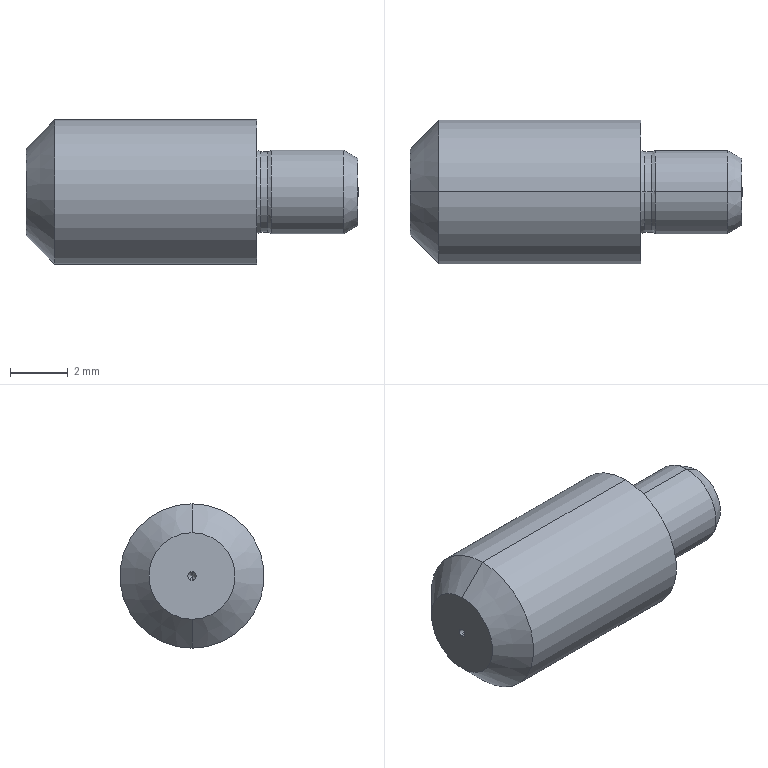Part | STEP file | kfsaph5_p2_90_l8_b3_0_e0_5_a30_2_03 | 1 solid | 21 faces | box 11.5 x 5 x 5 mm | volume 172.579 mm3 | cone 8 | cylinder 6 | spline 4 | plane 3 | commonest cylinder face diameters 2.8 x2 2.9 x2 5 x2
STEP:
#1=CARTESIAN_POINT('',(0.1323,0.,-1.4));
#2=VERTEX_POINT('',#1);
#3=CARTESIAN_POINT('',(0.1323,0.,1.4));
#4=VERTEX_POINT('',#3);
#5=CARTESIAN_POINT('',(0.1323,0.,0.));
#6=DIRECTION('',(1.,0.,0.));
#7=DIRECTION('',(0.,0.,1.));
#8=AXIS2_PLACEMENT_3D('',#5,#6,#7);
#9=CIRCLE('',#8,1.4);
#10=EDGE_CURVE('',#2,#4,#9,.T.);
#11=ORIENTED_EDGE('',*,*,#10,.F.);
#12=CARTESIAN_POINT('',(0.,0.,-1.45));
#13=VERTEX_POINT('',#12);
#14=CARTESIAN_POINT('',(0.1323,0.,-1.6));
#15=DIRECTION('',(0.,-1.,0.));
#16=DIRECTION('',(0.,0.,-1.));
#17=AXIS2_PLACEMENT_3D('',#14,#15,#16);
#18=CIRCLE('',#17,0.2);
#19=EDGE_CURVE('',#2,#13,#18,.T.);
#20=ORIENTED_EDGE('',*,*,#19,.T.);
#21=CARTESIAN_POINT('',(0.,0.,1.45));
#22=VERTEX_POINT('',#21);
#23=CARTESIAN_POINT('',(0.,0.,0.));
#24=DIRECTION('',(-1.,0.,0.));
#25=DIRECTION('',(0.,0.,1.));
#26=AXIS2_PLACEMENT_3D('',#23,#24,#25);
#27=CIRCLE('',#26,1.45);
#28=EDGE_CURVE('',#22,#13,#27,.T.);
#29=ORIENTED_EDGE('',*,*,#28,.F.);
#30=CARTESIAN_POINT('',(0.1323,0.,1.6));
#31=DIRECTION('',(0.,1.,0.));
#32=DIRECTION('',(0.,0.,1.));
#33=AXIS2_PLACEMENT_3D('',#30,#31,#32);
#34=CIRCLE('',#33,0.2);
#35=EDGE_CURVE('',#4,#22,#34,.T.);
#36=ORIENTED_EDGE('',*,*,#35,.F.);
#37=EDGE_LOOP('',(#11,#20,#29,#36));
#38=FACE_OUTER_BOUND('',#37,.T.);
#39=CARTESIAN_POINT('',(0.1323,0.,1.4));
#40=CARTESIAN_POINT('',(0.1323,2.8,1.4));
#41=CARTESIAN_POINT('',(0.1323,2.8,-1.4));
#42=CARTESIAN_POINT('',(0.1323,0.,-1.4));
#43=CARTESIAN_POINT('',(0.08303,0.,1.4));
#44=CARTESIAN_POINT('',(0.08303,2.8,1.4));
#45=CARTESIAN_POINT('',(0.08303,2.8,-1.4));
#46=CARTESIAN_POINT('',(0.08303,0.,-1.4));
#47=CARTESIAN_POINT('',(0.03695,0.,1.417));
#48=CARTESIAN_POINT('',(0.03695,2.835,1.417));
#49=CARTESIAN_POINT('',(0.03695,2.835,-1.417));
#50=CARTESIAN_POINT('',(0.03695,0.,-1.417));
#51=CARTESIAN_POINT('',(0.,0.,1.45));
#52=CARTESIAN_POINT('',(0.,2.9,1.45));
#53=CARTESIAN_POINT('',(0.,2.9,-1.45));
#54=CARTESIAN_POINT('',(0.,0.,-1.45));
#55=(BOUNDED_SURFACE()B_SPLINE_SURFACE(3,3,((#39,#40,#41,#42),(#43,#44,#45,#46),(#47,#48,#49,#50),(#51,#52,#53,#54)),.UNSPECIFIED.,.F.,.F.,.F.)B_SPLINE_SURFACE_WITH_KNOTS((4,4),(4,4),(0.,1.),(0.,1.),.UNSPECIFIED.)GEOMETRIC_REPRESENTATION_ITEM()RATIONAL_B_SPLINE_SURFACE(((1.,0.3333,0.3333,1.),(0.9569,0.319,0.319,0.9569),(0.9569,0.319,0.319,0.9569),(1.,0.3333,0.3333,1.)))REPRESENTATION_ITEM('')SURFACE());
#56=ADVANCED_FACE('',(#38),#55,.F.);
#57=CARTESIAN_POINT('',(0.5,0.,-1.45));
#58=VERTEX_POINT('',#57);
#59=CARTESIAN_POINT('',(0.5,0.,1.45));
#60=VERTEX_POINT('',#59);
#61=CARTESIAN_POINT('',(0.5,0.,0.));
#62=DIRECTION('',(1.,0.,0.));
#63=DIRECTION('',(0.,0.,1.));
#64=AXIS2_PLACEMENT_3D('',#61,#62,#63);
#65=CIRCLE('',#64,1.45);
#66=EDGE_CURVE('',#58,#60,#65,.T.);
#67=ORIENTED_EDGE('',*,*,#66,.F.);
#68=CARTESIAN_POINT('',(0.3677,0.,-1.4));
#69=VERTEX_POINT('',#68);
#70=CARTESIAN_POINT('',(0.3677,0.,-1.6));
#71=DIRECTION('',(0.,-1.,0.));
#72=DIRECTION('',(0.,0.,-1.));
#73=AXIS2_PLACEMENT_3D('',#70,#71,#72);
#74=CIRCLE('',#73,0.2);
#75=EDGE_CURVE('',#58,#69,#74,.T.);
#76=ORIENTED_EDGE('',*,*,#75,.T.);
#77=CARTESIAN_POINT('',(0.3677,0.,1.4));
#78=VERTEX_POINT('',#77);
#79=CARTESIAN_POINT('',(0.3677,0.,0.));
#80=DIRECTION('',(-1.,0.,0.));
#81=DIRECTION('',(0.,0.,-1.));
#82=AXIS2_PLACEMENT_3D('',#79,#80,#81);
#83=CIRCLE('',#82,1.4);
#84=EDGE_CURVE('',#78,#69,#83,.T.);
#85=ORIENTED_EDGE('',*,*,#84,.F.);
#86=CARTESIAN_POINT('',(0.3677,0.,1.6));
#87=DIRECTION('',(0.,1.,0.));
#88=DIRECTION('',(0.,0.,1.));
#89=AXIS2_PLACEMENT_3D('',#86,#87,#88);
#90=CIRCLE('',#89,0.2);
#91=EDGE_CURVE('',#60,#78,#90,.T.);
#92=ORIENTED_EDGE('',*,*,#91,.F.);
#93=EDGE_LOOP('',(#67,#76,#85,#92));
#94=FACE_OUTER_BOUND('',#93,.T.);
#95=CARTESIAN_POINT('',(0.5,0.,1.45));
#96=CARTESIAN_POINT('',(0.5,2.9,1.45));
#97=CARTESIAN_POINT('',(0.5,2.9,-1.45));
#98=CARTESIAN_POINT('',(0.5,0.,-1.45));
#99=CARTESIAN_POINT('',(0.4631,0.,1.417));
#100=CARTESIAN_POINT('',(0.4631,2.835,1.417));
#101=CARTESIAN_POINT('',(0.4631,2.835,-1.417));
#102=CARTESIAN_POINT('',(0.4631,0.,-1.417));
#103=CARTESIAN_POINT('',(0.417,0.,1.4));
#104=CARTESIAN_POINT('',(0.417,2.8,1.4));
#105=CARTESIAN_POINT('',(0.417,2.8,-1.4));
#106=CARTESIAN_POINT('',(0.417,0.,-1.4));
#107=CARTESIAN_POINT('',(0.3677,0.,1.4));
#108=CARTESIAN_POINT('',(0.3677,2.8,1.4));
#109=CARTESIAN_POINT('',(0.3677,2.8,-1.4));
#110=CARTESIAN_POINT('',(0.3677,0.,-1.4));
#111=(BOUNDED_SURFACE()B_SPLINE_SURFACE(3,3,((#95,#96,#97,#98),(#99,#100,#101,#102),(#103,#104,#105,#106),(#107,#108,#109,#110)),.UNSPECIFIED.,.F.,.F.,.F.)B_SPLINE_SURFACE_WITH_KNOTS((4,4),(4,4),(0.,1.),(0.,1.),.UNSPECIFIED.)GEOMETRIC_REPRESENTATION_ITEM()RATIONAL_B_SPLINE_SURFACE(((1.,0.3333,0.3333,1.),(0.9569,0.319,0.319,0.9569),(0.9569,0.319,0.319,0.9569),(1.,0.3333,0.3333,1.)))REPRESENTATION_ITEM('')SURFACE());
#112=ADVANCED_FACE('',(#94),#111,.F.);
#113=CARTESIAN_POINT('',(-7.,0.,-2.5));
#114=VERTEX_POINT('',#113);
#115=CARTESIAN_POINT('',(-7.,0.,2.5));
#116=VERTEX_POINT('',#115);
#117=CARTESIAN_POINT('',(-7.,0.,0.));
#118=DIRECTION('',(1.,0.,0.));
#119=DIRECTION('',(0.,0.,-1.));
#120=AXIS2_PLACEMENT_3D('',#117,#118,#119);
#121=CIRCLE('',#120,2.5);
#122=EDGE_CURVE('',#114,#116,#121,.T.);
#123=ORIENTED_EDGE('',*,*,#122,.T.);
#124=CARTESIAN_POINT('',(0.,0.,2.5));
#125=VERTEX_POINT('',#124);
#126=CARTESIAN_POINT('',(-3.5,0.,2.5));
#127=DIRECTION('',(1.,0.,0.));
#128=VECTOR('',#127,1000.);
#129=LINE('',#126,#128);
#130=EDGE_CURVE('',#116,#125,#129,.T.);
#131=ORIENTED_EDGE('',*,*,#130,.T.);
#132=CARTESIAN_POINT('',(0.,0.,-2.5));
#133=VERTEX_POINT('',#132);
#134=CARTESIAN_POINT('',(0.,0.,0.));
#135=DIRECTION('',(-1.,0.,0.));
#136=DIRECTION('',(0.,0.,-1.));
#137=AXIS2_PLACEMENT_3D('',#134,#135,#136);
#138=CIRCLE('',#137,2.5);
#139=EDGE_CURVE('',#125,#133,#138,.T.);
#140=ORIENTED_EDGE('',*,*,#139,.T.);
#141=CARTESIAN_POINT('',(-3.5,0.,-2.5));
#142=DIRECTION('',(1.,0.,0.));
#143=VECTOR('',#142,1000.);
#144=LINE('',#141,#143);
#145=EDGE_CURVE('',#114,#133,#144,.T.);
#146=ORIENTED_EDGE('',*,*,#145,.F.);
#147=EDGE_LOOP('',(#123,#131,#140,#146));
#148=FACE_OUTER_BOUND('',#147,.T.);
#149=CARTESIAN_POINT('',(-3.5,0.,0.));
#150=DIRECTION('',(1.,0.,0.));
#151=DIRECTION('',(0.,0.,-1.));
#152=AXIS2_PLACEMENT_3D('',#149,#150,#151);
#153=CYLINDRICAL_SURFACE('',#152,2.5);
#154=ADVANCED_FACE('',(#148),#153,.T.);
#155=CARTESIAN_POINT('',(-8.,0.,-1.5));
#156=VERTEX_POINT('',#155);
#157=CARTESIAN_POINT('',(-8.,0.,1.5));
#158=VERTEX_POINT('',#157);
#159=CARTESIAN_POINT('',(-8.,0.,0.));
#160=DIRECTION('',(1.,0.,0.));
#161=DIRECTION('',(0.,0.,-1.));
#162=AXIS2_PLACEMENT_3D('',#159,#160,#161);
#163=CIRCLE('',#162,1.5);
#164=EDGE_CURVE('',#156,#158,#163,.T.);
#165=ORIENTED_EDGE('',*,*,#164,.T.);
#166=CARTESIAN_POINT('',(-7.,0.,2.5));
#167=DIRECTION('',(0.7071,0.,0.7071));
#168=VECTOR('',#167,1000.);
#169=LINE('',#166,#168);
#170=EDGE_CURVE('',#158,#116,#169,.T.);
#171=ORIENTED_EDGE('',*,*,#170,.T.);
#172=ORIENTED_EDGE('',*,*,#122,.F.);
#173=CARTESIAN_POINT('',(-7.,0.,-2.5));
#174=DIRECTION('',(0.7071,0.,-0.7071));
#175=VECTOR('',#174,1000.);
#176=LINE('',#173,#175);
#177=EDGE_CURVE('',#156,#114,#176,.T.);
#178=ORIENTED_EDGE('',*,*,#177,.F.);
#179=EDGE_LOOP('',(#165,#171,#172,#178));
#180=FACE_OUTER_BOUND('',#179,.T.);
#181=CARTESIAN_POINT('',(-7.,0.,0.));
#182=DIRECTION('',(1.,0.,0.));
#183=DIRECTION('',(0.,0.,-1.));
#184=AXIS2_PLACEMENT_3D('',#181,#182,#183);
#185=CONICAL_SURFACE('',#184,2.5,0.7854);
#186=ADVANCED_FACE('',(#180),#185,.T.);
#187=CARTESIAN_POINT('',(-7.749,0.,0.));
#188=VERTEX_POINT('',#187);
#189=CARTESIAN_POINT('',(-8.,0.,0.145));
#190=VERTEX_POINT('',#189);
#191=CARTESIAN_POINT('',(-8.,0.,0.145));
#192=DIRECTION('',(-0.866,0.,0.5));
#193=VECTOR('',#192,1000.);
#194=LINE('',#191,#193);
#195=EDGE_CURVE('',#188,#190,#194,.T.);
#196=ORIENTED_EDGE('',*,*,#195,.F.);
#197=CARTESIAN_POINT('',(-8.,0.,-0.145));
#198=VERTEX_POINT('',#197);
#199=CARTESIAN_POINT('',(-8.,0.,-0.145));
#200=DIRECTION('',(-0.866,0.,-0.5));
#201=VECTOR('',#200,1000.);
#202=LINE('',#199,#201);
#203=EDGE_CURVE('',#188,#198,#202,.T.);
#204=ORIENTED_EDGE('',*,*,#203,.T.);
#205=CARTESIAN_POINT('',(-8.,0.,0.));
#206=DIRECTION('',(1.,0.,0.));
#207=DIRECTION('',(0.,0.,1.));
#208=AXIS2_PLACEMENT_3D('',#205,#206,#207);
#209=CIRCLE('',#208,0.145);
#210=EDGE_CURVE('',#190,#198,#209,.T.);
#211=ORIENTED_EDGE('',*,*,#210,.F.);
#212=EDGE_LOOP('',(#196,#204,#211));
#213=FACE_OUTER_BOUND('',#212,.T.);
#214=CARTESIAN_POINT('',(-8.,0.,0.));
#215=DIRECTION('',(-1.,0.,0.));
#216=DIRECTION('',(0.,0.,1.));
#217=AXIS2_PLACEMENT_3D('',#214,#215,#216);
#218=CONICAL_SURFACE('',#217,0.145,0.5236);
#219=ADVANCED_FACE('',(#213),#218,.F.);
#220=ORIENTED_EDGE('',*,*,#10,.T.);
#221=CARTESIAN_POINT('',(0.25,0.,1.4));
#222=DIRECTION('',(1.,0.,0.));
#223=VECTOR('',#222,1000.);
#224=LINE('',#221,#223);
#225=EDGE_CURVE('',#4,#78,#224,.T.);
#226=ORIENTED_EDGE('',*,*,#225,.T.);
#227=ORIENTED_EDGE('',*,*,#84,.T.);
#228=CARTESIAN_POINT('',(0.25,0.,-1.4));
#229=DIRECTION('',(1.,0.,0.));
#230=VECTOR('',#229,1000.);
#231=LINE('',#228,#230);
#232=EDGE_CURVE('',#2,#69,#231,.T.);
#233=ORIENTED_EDGE('',*,*,#232,.F.);
#234=EDGE_LOOP('',(#220,#226,#227,#233));
#235=FACE_OUTER_BOUND('',#234,.T.);
#236=CARTESIAN_POINT('',(0.25,0.,0.));
#237=DIRECTION('',(1.,0.,0.));
#238=DIRECTION('',(0.,0.,-1.));
#239=AXIS2_PLACEMENT_3D('',#236,#237,#238);
#240=CYLINDRICAL_SURFACE('',#239,1.4);
#241=ADVANCED_FACE('',(#235),#240,.T.);
#242=ORIENTED_EDGE('',*,*,#66,.T.);
#243=CARTESIAN_POINT('',(3.,0.,1.45));
#244=VERTEX_POINT('',#243);
#245=CARTESIAN_POINT('',(1.75,0.,1.45));
#246=DIRECTION('',(1.,0.,0.));
#247=VECTOR('',#246,1000.);
#248=LINE('',#245,#247);
#249=EDGE_CURVE('',#60,#244,#248,.T.);
#250=ORIENTED_EDGE('',*,*,#249,.T.);
#251=CARTESIAN_POINT('',(3.,0.,-1.45));
#252=VERTEX_POINT('',#251);
#253=CARTESIAN_POINT('',(3.,0.,0.));
#254=DIRECTION('',(-1.,0.,0.));
#255=DIRECTION('',(0.,0.,-1.));
#256=AXIS2_PLACEMENT_3D('',#253,#254,#255);
#257=CIRCLE('',#256,1.45);
#258=EDGE_CURVE('',#244,#252,#257,.T.);
#259=ORIENTED_EDGE('',*,*,#258,.T.);
#260=CARTESIAN_POINT('',(1.75,0.,-1.45));
#261=DIRECTION('',(1.,0.,0.));
#262=VECTOR('',#261,1000.);
#263=LINE('',#260,#262);
#264=EDGE_CURVE('',#58,#252,#263,.T.);
#265=ORIENTED_EDGE('',*,*,#264,.F.);
#266=EDGE_LOOP('',(#242,#250,#259,#265));
#267=FACE_OUTER_BOUND('',#266,.T.);
#268=CARTESIAN_POINT('',(1.75,0.,0.));
#269=DIRECTION('',(1.,0.,0.));
#270=DIRECTION('',(0.,0.,-1.));
#271=AXIS2_PLACEMENT_3D('',#268,#269,#270);
#272=CYLINDRICAL_SURFACE('',#271,1.45);
#273=ADVANCED_FACE('',(#267),#272,.T.);
#274=CARTESIAN_POINT('',(3.5,0.,1.161));
#275=VERTEX_POINT('',#274);
#276=CARTESIAN_POINT('',(3.5,0.,-1.161));
#277=VERTEX_POINT('',#276);
#278=CARTESIAN_POINT('',(3.5,0.,0.));
#279=DIRECTION('',(-1.,0.,0.));
#280=DIRECTION('',(0.,0.,1.));
#281=AXIS2_PLACEMENT_3D('',#278,#279,#280);
#282=CIRCLE('',#281,1.161);
#283=EDGE_CURVE('',#275,#277,#282,.T.);
#284=ORIENTED_EDGE('',*,*,#283,.T.);
#285=CARTESIAN_POINT('',(3.,0.,-1.45));
#286=DIRECTION('',(-0.866,0.,-0.5));
#287=VECTOR('',#286,1000.);
#288=LINE('',#285,#287);
#289=EDGE_CURVE('',#277,#252,#288,.T.);
#290=ORIENTED_EDGE('',*,*,#289,.T.);
#291=ORIENTED_EDGE('',*,*,#258,.F.);
#292=CARTESIAN_POINT('',(3.,0.,1.45));
#293=DIRECTION('',(-0.866,0.,0.5));
#294=VECTOR('',#293,1000.);
#295=LINE('',#292,#294);
#296=EDGE_CURVE('',#275,#244,#295,.T.);
#297=ORIENTED_EDGE('',*,*,#296,.F.);
#298=EDGE_LOOP('',(#284,#290,#291,#297));
#299=FACE_OUTER_BOUND('',#298,.T.);
#300=CARTESIAN_POINT('',(3.,0.,0.));
#301=DIRECTION('',(-1.,0.,0.));
#302=DIRECTION('',(0.,0.,1.));
#303=AXIS2_PLACEMENT_3D('',#300,#301,#302);
#304=CONICAL_SURFACE('',#303,1.45,0.5236);
#305=ADVANCED_FACE('',(#299),#304,.T.);
#306=CARTESIAN_POINT('',(3.249,0.,0.));
#307=VERTEX_POINT('',#306);
#308=CARTESIAN_POINT('',(3.5,0.,-0.145));
#309=VERTEX_POINT('',#308);
#310=CARTESIAN_POINT('',(3.5,0.,-0.145));
#311=DIRECTION('',(0.866,0.,-0.5));
#312=VECTOR('',#311,1000.);
#313=LINE('',#310,#312);
#314=EDGE_CURVE('',#307,#309,#313,.T.);
#315=ORIENTED_EDGE('',*,*,#314,.F.);
#316=CARTESIAN_POINT('',(3.5,0.,0.145));
#317=VERTEX_POINT('',#316);
#318=CARTESIAN_POINT('',(3.5,0.,0.145));
#319=DIRECTION('',(0.866,0.,0.5));
#320=VECTOR('',#319,1000.);
#321=LINE('',#318,#320);
#322=EDGE_CURVE('',#307,#317,#321,.T.);
#323=ORIENTED_EDGE('',*,*,#322,.T.);
#324=CARTESIAN_POINT('',(3.5,0.,0.));
#325=DIRECTION('',(-1.,0.,0.));
#326=DIRECTION('',(0.,0.,-1.));
#327=AXIS2_PLACEMENT_3D('',#324,#325,#326);
#328=CIRCLE('',#327,0.145);
#329=EDGE_CURVE('',#309,#317,#328,.T.);
#330=ORIENTED_EDGE('',*,*,#329,.F.);
#331=EDGE_LOOP('',(#315,#323,#330));
#332=FACE_OUTER_BOUND('',#331,.T.);
#333=CARTESIAN_POINT('',(3.5,0.,0.));
#334=DIRECTION('',(1.,0.,0.));
#335=DIRECTION('',(0.,0.,-1.));
#336=AXIS2_PLACEMENT_3D('',#333,#334,#335);
#337=CONICAL_SURFACE('',#336,0.145,0.5236);
#338=ADVANCED_FACE('',(#332),#337,.F.);
#339=ORIENTED_EDGE('',*,*,#130,.F.);
#340=CARTESIAN_POINT('',(-7.,0.,0.));
#341=DIRECTION('',(1.,0.,0.));
#342=DIRECTION('',(0.,0.,-1.));
#343=AXIS2_PLACEMENT_3D('',#340,#341,#342);
#344=CIRCLE('',#343,2.5);
#345=EDGE_CURVE('',#116,#114,#344,.T.);
#346=ORIENTED_EDGE('',*,*,#345,.T.);
#347=ORIENTED_EDGE('',*,*,#145,.T.);
#348=CARTESIAN_POINT('',(0.,0.,0.));
#349=DIRECTION('',(-1.,0.,0.));
#350=DIRECTION('',(0.,0.,-1.));
#351=AXIS2_PLACEMENT_3D('',#348,#349,#350);
#352=CIRCLE('',#351,2.5);
#353=EDGE_CURVE('',#133,#125,#352,.T.);
#354=ORIENTED_EDGE('',*,*,#353,.T.);
#355=EDGE_LOOP('',(#339,#346,#347,#354));
#356=FACE_OUTER_BOUND('',#355,.T.);
#357=CARTESIAN_POINT('',(-3.5,0.,0.));
#358=DIRECTION('',(1.,0.,0.));
#359=DIRECTION('',(0.,0.,-1.));
#360=AXIS2_PLACEMENT_3D('',#357,#358,#359);
#361=CYLINDRICAL_SURFACE('',#360,2.5);
#362=ADVANCED_FACE('',(#356),#361,.T.);
#363=ORIENTED_EDGE('',*,*,#170,.F.);
#364=CARTESIAN_POINT('',(-8.,0.,0.));
#365=DIRECTION('',(1.,0.,0.));
#366=DIRECTION('',(0.,0.,-1.));
#367=AXIS2_PLACEMENT_3D('',#364,#365,#366);
#368=CIRCLE('',#367,1.5);
#369=EDGE_CURVE('',#158,#156,#368,.T.);
#370=ORIENTED_EDGE('',*,*,#369,.T.);
#371=ORIENTED_EDGE('',*,*,#177,.T.);
#372=ORIENTED_EDGE('',*,*,#345,.F.);
#373=EDGE_LOOP('',(#363,#370,#371,#372));
#374=FACE_OUTER_BOUND('',#373,.T.);
#375=CARTESIAN_POINT('',(-7.,0.,0.));
#376=DIRECTION('',(1.,0.,0.));
#377=DIRECTION('',(0.,0.,-1.));
#378=AXIS2_PLACEMENT_3D('',#375,#376,#377);
#379=CONICAL_SURFACE('',#378,2.5,0.7854);
#380=ADVANCED_FACE('',(#374),#379,.T.);
#381=ORIENTED_EDGE('',*,*,#353,.F.);
#382=ORIENTED_EDGE('',*,*,#139,.F.);
#383=EDGE_LOOP('',(#381,#382));
#384=FACE_OUTER_BOUND('',#383,.T.);
#385=ORIENTED_EDGE('',*,*,#28,.T.);
#386=CARTESIAN_POINT('',(0.,0.,0.));
#387=DIRECTION('',(-1.,0.,0.));
#388=DIRECTION('',(0.,0.,1.));
#389=AXIS2_PLACEMENT_3D('',#386,#387,#388);
#390=CIRCLE('',#389,1.45);
#391=EDGE_CURVE('',#13,#22,#390,.T.);
#392=ORIENTED_EDGE('',*,*,#391,.T.);
#393=EDGE_LOOP('',(#385,#392));
#394=FACE_BOUND('',#393,.T.);
#395=CARTESIAN_POINT('',(0.,1.25,0.));
#396=DIRECTION('',(1.,0.,0.));
#397=DIRECTION('',(0.,0.,-1.));
#398=AXIS2_PLACEMENT_3D('',#395,#396,#397);
#399=PLANE('',#398);
#400=ADVANCED_FACE('',(#384,#394),#399,.T.);
#401=ORIENTED_EDGE('',*,*,#164,.F.);
#402=ORIENTED_EDGE('',*,*,#369,.F.);
#403=EDGE_LOOP('',(#401,#402));
#404=FACE_OUTER_BOUND('',#403,.T.);
#405=ORIENTED_EDGE('',*,*,#210,.T.);
#406=CARTESIAN_POINT('',(-8.,0.,0.));
#407=DIRECTION('',(1.,0.,0.));
#408=DIRECTION('',(0.,0.,1.));
#409=AXIS2_PLACEMENT_3D('',#406,#407,#408);
#410=CIRCLE('',#409,0.145);
#411=EDGE_CURVE('',#198,#190,#410,.T.);
#412=ORIENTED_EDGE('',*,*,#411,.T.);
#413=EDGE_LOOP('',(#405,#412));
#414=FACE_BOUND('',#413,.T.);
#415=CARTESIAN_POINT('',(-8.,0.8225,0.));
#416=DIRECTION('',(-1.,0.,0.));
#417=DIRECTION('',(0.,0.,1.));
#418=AXIS2_PLACEMENT_3D('',#415,#416,#417);
#419=PLANE('',#418);
#420=ADVANCED_FACE('',(#404,#414),#419,.T.);
#421=ORIENTED_EDGE('',*,*,#19,.F.);
#422=CARTESIAN_POINT('',(0.1323,0.,0.));
#423=DIRECTION('',(1.,0.,0.));
#424=DIRECTION('',(0.,0.,1.));
#425=AXIS2_PLACEMENT_3D('',#422,#423,#424);
#426=CIRCLE('',#425,1.4);
#427=EDGE_CURVE('',#4,#2,#426,.T.);
#428=ORIENTED_EDGE('',*,*,#427,.F.);
#429=ORIENTED_EDGE('',*,*,#35,.T.);
#430=ORIENTED_EDGE('',*,*,#391,.F.);
#431=EDGE_LOOP('',(#421,#428,#429,#430));
#432=FACE_OUTER_BOUND('',#431,.T.);
#433=CARTESIAN_POINT('',(0.1323,0.,-1.4));
#434=CARTESIAN_POINT('',(0.1323,-2.8,-1.4));
#435=CARTESIAN_POINT('',(0.1323,-2.8,1.4));
#436=CARTESIAN_POINT('',(0.1323,0.,1.4));
#437=CARTESIAN_POINT('',(0.08303,0.,-1.4));
#438=CARTESIAN_POINT('',(0.08303,-2.8,-1.4));
#439=CARTESIAN_POINT('',(0.08303,-2.8,1.4));
#440=CARTESIAN_POINT('',(0.08303,0.,1.4));
#441=CARTESIAN_POINT('',(0.03695,0.,-1.417));
#442=CARTESIAN_POINT('',(0.03695,-2.835,-1.417));
#443=CARTESIAN_POINT('',(0.03695,-2.835,1.417));
#444=CARTESIAN_POINT('',(0.03695,0.,1.417));
#445=CARTESIAN_POINT('',(0.,0.,-1.45));
#446=CARTESIAN_POINT('',(0.,-2.9,-1.45));
#447=CARTESIAN_POINT('',(0.,-2.9,1.45));
#448=CARTESIAN_POINT('',(0.,0.,1.45));
#449=(BOUNDED_SURFACE()B_SPLINE_SURFACE(3,3,((#433,#434,#435,#436),(#437,#438,#439,#440),(#441,#442,#443,#444),(#445,#446,#447,#448)),.UNSPECIFIED.,.F.,.F.,.F.)B_SPLINE_SURFACE_WITH_KNOTS((4,4),(4,4),(0.,1.),(0.,1.),.UNSPECIFIED.)GEOMETRIC_REPRESENTATION_ITEM()RATIONAL_B_SPLINE_SURFACE(((1.,0.3333,0.3333,1.),(0.9569,0.319,0.319,0.9569),(0.9569,0.319,0.319,0.9569),(1.,0.3333,0.3333,1.)))REPRESENTATION_ITEM('')SURFACE());
#450=ADVANCED_FACE('',(#432),#449,.F.);
#451=ORIENTED_EDGE('',*,*,#203,.F.);
#452=ORIENTED_EDGE('',*,*,#195,.T.);
#453=ORIENTED_EDGE('',*,*,#411,.F.);
#454=EDGE_LOOP('',(#451,#452,#453));
#455=FACE_OUTER_BOUND('',#454,.T.);
#456=CARTESIAN_POINT('',(-8.,0.,0.));
#457=DIRECTION('',(-1.,0.,0.));
#458=DIRECTION('',(0.,0.,1.));
#459=AXIS2_PLACEMENT_3D('',#456,#457,#458);
#460=CONICAL_SURFACE('',#459,0.145,0.5236);
#461=ADVANCED_FACE('',(#455),#460,.F.);
#462=ORIENTED_EDGE('',*,*,#225,.F.);
#463=ORIENTED_EDGE('',*,*,#427,.T.);
#464=ORIENTED_EDGE('',*,*,#232,.T.);
#465=CARTESIAN_POINT('',(0.3677,0.,0.));
#466=DIRECTION('',(-1.,0.,0.));
#467=DIRECTION('',(0.,0.,-1.));
#468=AXIS2_PLACEMENT_3D('',#465,#466,#467);
#469=CIRCLE('',#468,1.4);
#470=EDGE_CURVE('',#69,#78,#469,.T.);
#471=ORIENTED_EDGE('',*,*,#470,.T.);
#472=EDGE_LOOP('',(#462,#463,#464,#471));
#473=FACE_OUTER_BOUND('',#472,.T.);
#474=CARTESIAN_POINT('',(0.25,0.,0.));
#475=DIRECTION('',(1.,0.,0.));
#476=DIRECTION('',(0.,0.,-1.));
#477=AXIS2_PLACEMENT_3D('',#474,#475,#476);
#478=CYLINDRICAL_SURFACE('',#477,1.4);
#479=ADVANCED_FACE('',(#473),#478,.T.);
#480=ORIENTED_EDGE('',*,*,#75,.F.);
#481=CARTESIAN_POINT('',(0.5,0.,0.));
#482=DIRECTION('',(1.,0.,0.));
#483=DIRECTION('',(0.,0.,1.));
#484=AXIS2_PLACEMENT_3D('',#481,#482,#483);
#485=CIRCLE('',#484,1.45);
#486=EDGE_CURVE('',#60,#58,#485,.T.);
#487=ORIENTED_EDGE('',*,*,#486,.F.);
#488=ORIENTED_EDGE('',*,*,#91,.T.);
#489=ORIENTED_EDGE('',*,*,#470,.F.);
#490=EDGE_LOOP('',(#480,#487,#488,#489));
#491=FACE_OUTER_BOUND('',#490,.T.);
#492=CARTESIAN_POINT('',(0.5,0.,-1.45));
#493=CARTESIAN_POINT('',(0.5,-2.9,-1.45));
#494=CARTESIAN_POINT('',(0.5,-2.9,1.45));
#495=CARTESIAN_POINT('',(0.5,0.,1.45));
#496=CARTESIAN_POINT('',(0.4631,0.,-1.417));
#497=CARTESIAN_POINT('',(0.4631,-2.835,-1.417));
#498=CARTESIAN_POINT('',(0.4631,-2.835,1.417));
#499=CARTESIAN_POINT('',(0.4631,0.,1.417));
#500=CARTESIAN_POINT('',(0.417,0.,-1.4));
#501=CARTESIAN_POINT('',(0.417,-2.8,-1.4));
#502=CARTESIAN_POINT('',(0.417,-2.8,1.4));
#503=CARTESIAN_POINT('',(0.417,0.,1.4));
#504=CARTESIAN_POINT('',(0.3677,0.,-1.4));
#505=CARTESIAN_POINT('',(0.3677,-2.8,-1.4));
#506=CARTESIAN_POINT('',(0.3677,-2.8,1.4));
#507=CARTESIAN_POINT('',(0.3677,0.,1.4));
#508=(BOUNDED_SURFACE()B_SPLINE_SURFACE(3,3,((#492,#493,#494,#495),(#496,#497,#498,#499),(#500,#501,#502,#503),(#504,#505,#506,#507)),.UNSPECIFIED.,.F.,.F.,.F.)B_SPLINE_SURFACE_WITH_KNOTS((4,4),(4,4),(0.,1.),(0.,1.),.UNSPECIFIED.)GEOMETRIC_REPRESENTATION_ITEM()RATIONAL_B_SPLINE_SURFACE(((1.,0.3333,0.3333,1.),(0.9569,0.319,0.319,0.9569),(0.9569,0.319,0.319,0.9569),(1.,0.3333,0.3333,1.)))REPRESENTATION_ITEM('')SURFACE());
#509=ADVANCED_FACE('',(#491),#508,.F.);
#510=ORIENTED_EDGE('',*,*,#249,.F.);
#511=ORIENTED_EDGE('',*,*,#486,.T.);
#512=ORIENTED_EDGE('',*,*,#264,.T.);
#513=CARTESIAN_POINT('',(3.,0.,0.));
#514=DIRECTION('',(-1.,0.,0.));
#515=DIRECTION('',(0.,0.,-1.));
#516=AXIS2_PLACEMENT_3D('',#513,#514,#515);
#517=CIRCLE('',#516,1.45);
#518=EDGE_CURVE('',#252,#244,#517,.T.);
#519=ORIENTED_EDGE('',*,*,#518,.T.);
#520=EDGE_LOOP('',(#510,#511,#512,#519));
#521=FACE_OUTER_BOUND('',#520,.T.);
#522=CARTESIAN_POINT('',(1.75,0.,0.));
#523=DIRECTION('',(1.,0.,0.));
#524=DIRECTION('',(0.,0.,-1.));
#525=AXIS2_PLACEMENT_3D('',#522,#523,#524);
#526=CYLINDRICAL_SURFACE('',#525,1.45);
#527=ADVANCED_FACE('',(#521),#526,.T.);
#528=ORIENTED_EDGE('',*,*,#289,.F.);
#529=CARTESIAN_POINT('',(3.5,0.,0.));
#530=DIRECTION('',(-1.,0.,0.));
#531=DIRECTION('',(0.,0.,1.));
#532=AXIS2_PLACEMENT_3D('',#529,#530,#531);
#533=CIRCLE('',#532,1.161);
#534=EDGE_CURVE('',#277,#275,#533,.T.);
#535=ORIENTED_EDGE('',*,*,#534,.T.);
#536=ORIENTED_EDGE('',*,*,#296,.T.);
#537=ORIENTED_EDGE('',*,*,#518,.F.);
#538=EDGE_LOOP('',(#528,#535,#536,#537));
#539=FACE_OUTER_BOUND('',#538,.T.);
#540=CARTESIAN_POINT('',(3.,0.,0.));
#541=DIRECTION('',(-1.,0.,0.));
#542=DIRECTION('',(0.,0.,1.));
#543=AXIS2_PLACEMENT_3D('',#540,#541,#542);
#544=CONICAL_SURFACE('',#543,1.45,0.5236);
#545=ADVANCED_FACE('',(#539),#544,.T.);
#546=ORIENTED_EDGE('',*,*,#329,.T.);
#547=CARTESIAN_POINT('',(3.5,0.,0.));
#548=DIRECTION('',(-1.,0.,0.));
#549=DIRECTION('',(0.,0.,-1.));
#550=AXIS2_PLACEMENT_3D('',#547,#548,#549);
#551=CIRCLE('',#550,0.145);
#552=EDGE_CURVE('',#317,#309,#551,.T.);
#553=ORIENTED_EDGE('',*,*,#552,.T.);
#554=EDGE_LOOP('',(#546,#553));
#555=FACE_BOUND('',#554,.T.);
#556=ORIENTED_EDGE('',*,*,#283,.F.);
#557=ORIENTED_EDGE('',*,*,#534,.F.);
#558=EDGE_LOOP('',(#556,#557));
#559=FACE_OUTER_BOUND('',#558,.T.);
#560=CARTESIAN_POINT('',(3.5,0.6532,0.));
#561=DIRECTION('',(1.,0.,0.));
#562=DIRECTION('',(0.,0.,-1.));
#563=AXIS2_PLACEMENT_3D('',#560,#561,#562);
#564=PLANE('',#563);
#565=ADVANCED_FACE('',(#555,#559),#564,.T.);
#566=ORIENTED_EDGE('',*,*,#322,.F.);
#567=ORIENTED_EDGE('',*,*,#314,.T.);
#568=ORIENTED_EDGE('',*,*,#552,.F.);
#569=EDGE_LOOP('',(#566,#567,#568));
#570=FACE_OUTER_BOUND('',#569,.T.);
#571=CARTESIAN_POINT('',(3.5,0.,0.));
#572=DIRECTION('',(1.,0.,0.));
#573=DIRECTION('',(0.,0.,-1.));
#574=AXIS2_PLACEMENT_3D('',#571,#572,#573);
#575=CONICAL_SURFACE('',#574,0.145,0.5236);
#576=ADVANCED_FACE('',(#570),#575,.F.);
#577=CLOSED_SHELL('',(#56,#112,#154,#186,#219,#241,#273,#305,#338,#362,#380,#400,#420,#450,#461,#479,#509,#527,#545,#565,#576));
#578=MANIFOLD_SOLID_BREP('',#577);
#579=CARTESIAN_POINT('',(0.,0.,0.));
#580=DIRECTION('',(0.,0.,1.));
#581=DIRECTION('',(1.,0.,0.));
#582=AXIS2_PLACEMENT_3D('',#579,#580,#581);
#583=(LENGTH_UNIT()NAMED_UNIT(*)SI_UNIT(.MILLI.,.METRE.));
#584=UNCERTAINTY_MEASURE_WITH_UNIT(LENGTH_MEASURE(0.00001),#583,'','');
#585=(NAMED_UNIT(*)PLANE_ANGLE_UNIT()SI_UNIT($,.RADIAN.));
#586=(NAMED_UNIT(*)SI_UNIT($,.STERADIAN.)SOLID_ANGLE_UNIT());
#587=(GEOMETRIC_REPRESENTATION_CONTEXT(3)GLOBAL_UNCERTAINTY_ASSIGNED_CONTEXT((#584))GLOBAL_UNIT_ASSIGNED_CONTEXT((#583,#585,#586))REPRESENTATION_CONTEXT('',''));
#588=ADVANCED_BREP_SHAPE_REPRESENTATION('',(#578,#582),#587);